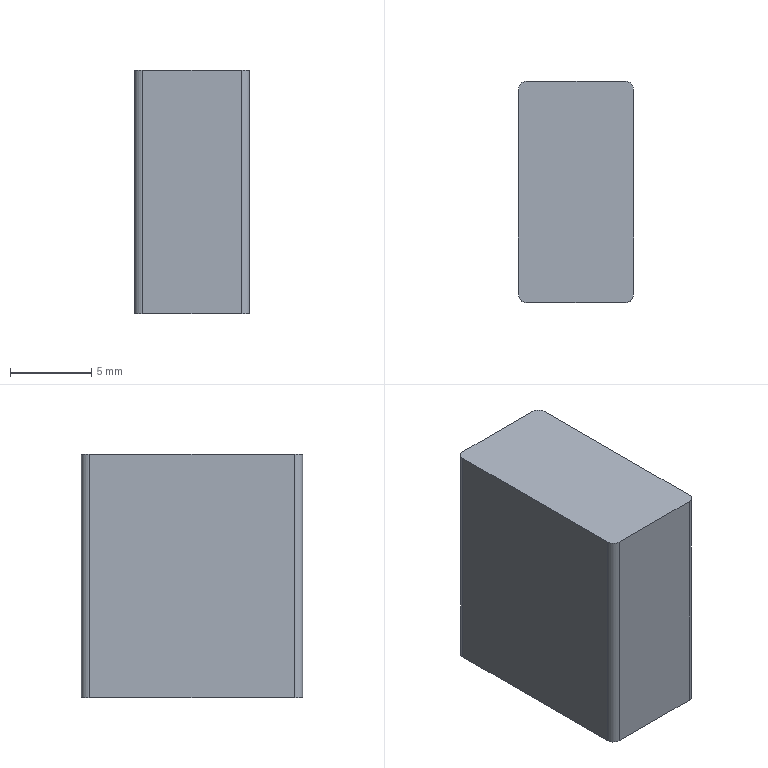Part | NX | features BREP 1 | 1 solid | 10 faces | box 7.1 x 13.637 x 15 mm | volume 1449 mm3 | plane 6 | cylinder 4 | commonest cylinder face diameters 1 x4
STEP:
#1=CARTESIAN_POINT('',(-3.05,6.819,-25.6));
#2=VERTEX_POINT('',#1);
#3=CARTESIAN_POINT('',(-3.55,6.319,-25.6));
#4=VERTEX_POINT('',#3);
#5=CARTESIAN_POINT('',(-3.05,6.319,-25.6));
#6=DIRECTION('',(0.,0.,1.));
#7=DIRECTION('',(1.,0.,0.));
#8=AXIS2_PLACEMENT_3D('',#5,#6,#7);
#9=CIRCLE('',#8,0.5);
#10=EDGE_CURVE('',#2,#4,#9,.T.);
#11=ORIENTED_EDGE('',*,*,#10,.F.);
#12=CARTESIAN_POINT('',(-3.05,6.819,-40.6));
#13=VERTEX_POINT('',#12);
#14=CARTESIAN_POINT('',(-3.05,6.819,-40.6));
#15=DIRECTION('',(0.,0.,1.));
#16=VECTOR('',#15,1000.);
#17=LINE('',#14,#16);
#18=EDGE_CURVE('',#13,#2,#17,.T.);
#19=ORIENTED_EDGE('',*,*,#18,.F.);
#20=CARTESIAN_POINT('',(-3.55,6.319,-40.6));
#21=VERTEX_POINT('',#20);
#22=CARTESIAN_POINT('',(-3.05,6.319,-40.6));
#23=DIRECTION('',(0.,0.,1.));
#24=DIRECTION('',(1.,0.,0.));
#25=AXIS2_PLACEMENT_3D('',#22,#23,#24);
#26=CIRCLE('',#25,0.5);
#27=EDGE_CURVE('',#13,#21,#26,.T.);
#28=ORIENTED_EDGE('',*,*,#27,.T.);
#29=CARTESIAN_POINT('',(-3.55,6.319,-40.6));
#30=DIRECTION('',(0.,0.,1.));
#31=VECTOR('',#30,1000.);
#32=LINE('',#29,#31);
#33=EDGE_CURVE('',#21,#4,#32,.T.);
#34=ORIENTED_EDGE('',*,*,#33,.T.);
#35=EDGE_LOOP('',(#11,#19,#28,#34));
#36=FACE_BOUND('',#35,.T.);
#37=CARTESIAN_POINT('',(-3.05,6.319,-40.6));
#38=DIRECTION('',(0.,0.,1.));
#39=DIRECTION('',(-1.,0.,0.));
#40=AXIS2_PLACEMENT_3D('',#37,#38,#39);
#41=CYLINDRICAL_SURFACE('',#40,0.5);
#42=ADVANCED_FACE('',(#36),#41,.T.);
#43=CARTESIAN_POINT('',(-3.55,-6.319,-25.6));
#44=VERTEX_POINT('',#43);
#45=CARTESIAN_POINT('',(-3.55,-6.319,-25.6));
#46=DIRECTION('',(0.,1.,0.));
#47=VECTOR('',#46,1000.);
#48=LINE('',#45,#47);
#49=EDGE_CURVE('',#44,#4,#48,.T.);
#50=ORIENTED_EDGE('',*,*,#49,.T.);
#51=ORIENTED_EDGE('',*,*,#33,.F.);
#52=CARTESIAN_POINT('',(-3.55,-6.319,-40.6));
#53=VERTEX_POINT('',#52);
#54=CARTESIAN_POINT('',(-3.55,-6.319,-40.6));
#55=DIRECTION('',(0.,1.,0.));
#56=VECTOR('',#55,1000.);
#57=LINE('',#54,#56);
#58=EDGE_CURVE('',#53,#21,#57,.T.);
#59=ORIENTED_EDGE('',*,*,#58,.F.);
#60=CARTESIAN_POINT('',(-3.55,-6.319,-40.6));
#61=DIRECTION('',(0.,0.,1.));
#62=VECTOR('',#61,1000.);
#63=LINE('',#60,#62);
#64=EDGE_CURVE('',#53,#44,#63,.T.);
#65=ORIENTED_EDGE('',*,*,#64,.T.);
#66=EDGE_LOOP('',(#50,#51,#59,#65));
#67=FACE_BOUND('',#66,.T.);
#68=CARTESIAN_POINT('',(-3.55,-6.319,-40.6));
#69=DIRECTION('',(1.,0.,0.));
#70=DIRECTION('',(0.,-1.,0.));
#71=AXIS2_PLACEMENT_3D('',#68,#69,#70);
#72=PLANE('',#71);
#73=ADVANCED_FACE('',(#67),#72,.F.);
#74=CARTESIAN_POINT('',(-3.05,-6.819,-25.6));
#75=VERTEX_POINT('',#74);
#76=CARTESIAN_POINT('',(-3.05,-6.319,-25.6));
#77=DIRECTION('',(0.,0.,1.));
#78=DIRECTION('',(1.,0.,0.));
#79=AXIS2_PLACEMENT_3D('',#76,#77,#78);
#80=CIRCLE('',#79,0.5);
#81=EDGE_CURVE('',#44,#75,#80,.T.);
#82=ORIENTED_EDGE('',*,*,#81,.F.);
#83=ORIENTED_EDGE('',*,*,#64,.F.);
#84=CARTESIAN_POINT('',(-3.05,-6.819,-40.6));
#85=VERTEX_POINT('',#84);
#86=CARTESIAN_POINT('',(-3.05,-6.319,-40.6));
#87=DIRECTION('',(0.,0.,1.));
#88=DIRECTION('',(1.,0.,0.));
#89=AXIS2_PLACEMENT_3D('',#86,#87,#88);
#90=CIRCLE('',#89,0.5);
#91=EDGE_CURVE('',#53,#85,#90,.T.);
#92=ORIENTED_EDGE('',*,*,#91,.T.);
#93=CARTESIAN_POINT('',(-3.05,-6.819,-40.6));
#94=DIRECTION('',(0.,0.,1.));
#95=VECTOR('',#94,1000.);
#96=LINE('',#93,#95);
#97=EDGE_CURVE('',#85,#75,#96,.T.);
#98=ORIENTED_EDGE('',*,*,#97,.T.);
#99=EDGE_LOOP('',(#82,#83,#92,#98));
#100=FACE_BOUND('',#99,.T.);
#101=CARTESIAN_POINT('',(-3.05,-6.319,-40.6));
#102=DIRECTION('',(0.,0.,1.));
#103=DIRECTION('',(-1.,0.,0.));
#104=AXIS2_PLACEMENT_3D('',#101,#102,#103);
#105=CYLINDRICAL_SURFACE('',#104,0.5);
#106=ADVANCED_FACE('',(#100),#105,.T.);
#107=CARTESIAN_POINT('',(3.05,-6.819,-25.6));
#108=VERTEX_POINT('',#107);
#109=CARTESIAN_POINT('',(3.05,-6.819,-25.6));
#110=DIRECTION('',(-1.,0.,0.));
#111=VECTOR('',#110,1000.);
#112=LINE('',#109,#111);
#113=EDGE_CURVE('',#108,#75,#112,.T.);
#114=ORIENTED_EDGE('',*,*,#113,.T.);
#115=ORIENTED_EDGE('',*,*,#97,.F.);
#116=CARTESIAN_POINT('',(3.05,-6.819,-40.6));
#117=VERTEX_POINT('',#116);
#118=CARTESIAN_POINT('',(3.05,-6.819,-40.6));
#119=DIRECTION('',(-1.,0.,0.));
#120=VECTOR('',#119,1000.);
#121=LINE('',#118,#120);
#122=EDGE_CURVE('',#117,#85,#121,.T.);
#123=ORIENTED_EDGE('',*,*,#122,.F.);
#124=CARTESIAN_POINT('',(3.05,-6.819,-40.6));
#125=DIRECTION('',(0.,0.,1.));
#126=VECTOR('',#125,1000.);
#127=LINE('',#124,#126);
#128=EDGE_CURVE('',#117,#108,#127,.T.);
#129=ORIENTED_EDGE('',*,*,#128,.T.);
#130=EDGE_LOOP('',(#114,#115,#123,#129));
#131=FACE_BOUND('',#130,.T.);
#132=CARTESIAN_POINT('',(3.05,-6.819,-40.6));
#133=DIRECTION('',(0.,1.,0.));
#134=DIRECTION('',(0.,0.,-1.));
#135=AXIS2_PLACEMENT_3D('',#132,#133,#134);
#136=PLANE('',#135);
#137=ADVANCED_FACE('',(#131),#136,.F.);
#138=CARTESIAN_POINT('',(3.55,-6.319,-25.6));
#139=VERTEX_POINT('',#138);
#140=CARTESIAN_POINT('',(3.05,-6.319,-25.6));
#141=DIRECTION('',(0.,0.,1.));
#142=DIRECTION('',(1.,0.,0.));
#143=AXIS2_PLACEMENT_3D('',#140,#141,#142);
#144=CIRCLE('',#143,0.5);
#145=EDGE_CURVE('',#108,#139,#144,.T.);
#146=ORIENTED_EDGE('',*,*,#145,.F.);
#147=ORIENTED_EDGE('',*,*,#128,.F.);
#148=CARTESIAN_POINT('',(3.55,-6.319,-40.6));
#149=VERTEX_POINT('',#148);
#150=CARTESIAN_POINT('',(3.05,-6.319,-40.6));
#151=DIRECTION('',(0.,0.,1.));
#152=DIRECTION('',(1.,0.,0.));
#153=AXIS2_PLACEMENT_3D('',#150,#151,#152);
#154=CIRCLE('',#153,0.5);
#155=EDGE_CURVE('',#117,#149,#154,.T.);
#156=ORIENTED_EDGE('',*,*,#155,.T.);
#157=CARTESIAN_POINT('',(3.55,-6.319,-40.6));
#158=DIRECTION('',(0.,0.,1.));
#159=VECTOR('',#158,1000.);
#160=LINE('',#157,#159);
#161=EDGE_CURVE('',#149,#139,#160,.T.);
#162=ORIENTED_EDGE('',*,*,#161,.T.);
#163=EDGE_LOOP('',(#146,#147,#156,#162));
#164=FACE_BOUND('',#163,.T.);
#165=CARTESIAN_POINT('',(3.05,-6.319,-40.6));
#166=DIRECTION('',(0.,0.,1.));
#167=DIRECTION('',(-1.,0.,0.));
#168=AXIS2_PLACEMENT_3D('',#165,#166,#167);
#169=CYLINDRICAL_SURFACE('',#168,0.5);
#170=ADVANCED_FACE('',(#164),#169,.T.);
#171=CARTESIAN_POINT('',(3.55,6.319,-25.6));
#172=VERTEX_POINT('',#171);
#173=CARTESIAN_POINT('',(3.55,6.319,-25.6));
#174=DIRECTION('',(0.,-1.,0.));
#175=VECTOR('',#174,1000.);
#176=LINE('',#173,#175);
#177=EDGE_CURVE('',#172,#139,#176,.T.);
#178=ORIENTED_EDGE('',*,*,#177,.T.);
#179=ORIENTED_EDGE('',*,*,#161,.F.);
#180=CARTESIAN_POINT('',(3.55,6.319,-40.6));
#181=VERTEX_POINT('',#180);
#182=CARTESIAN_POINT('',(3.55,6.319,-40.6));
#183=DIRECTION('',(0.,-1.,0.));
#184=VECTOR('',#183,1000.);
#185=LINE('',#182,#184);
#186=EDGE_CURVE('',#181,#149,#185,.T.);
#187=ORIENTED_EDGE('',*,*,#186,.F.);
#188=CARTESIAN_POINT('',(3.55,6.319,-40.6));
#189=DIRECTION('',(0.,0.,1.));
#190=VECTOR('',#189,1000.);
#191=LINE('',#188,#190);
#192=EDGE_CURVE('',#181,#172,#191,.T.);
#193=ORIENTED_EDGE('',*,*,#192,.T.);
#194=EDGE_LOOP('',(#178,#179,#187,#193));
#195=FACE_BOUND('',#194,.T.);
#196=CARTESIAN_POINT('',(3.55,6.319,-40.6));
#197=DIRECTION('',(-1.,0.,0.));
#198=DIRECTION('',(0.,1.,0.));
#199=AXIS2_PLACEMENT_3D('',#196,#197,#198);
#200=PLANE('',#199);
#201=ADVANCED_FACE('',(#195),#200,.F.);
#202=CARTESIAN_POINT('',(3.05,6.819,-25.6));
#203=VERTEX_POINT('',#202);
#204=CARTESIAN_POINT('',(3.05,6.319,-25.6));
#205=DIRECTION('',(0.,0.,1.));
#206=DIRECTION('',(1.,0.,0.));
#207=AXIS2_PLACEMENT_3D('',#204,#205,#206);
#208=CIRCLE('',#207,0.5);
#209=EDGE_CURVE('',#172,#203,#208,.T.);
#210=ORIENTED_EDGE('',*,*,#209,.F.);
#211=ORIENTED_EDGE('',*,*,#192,.F.);
#212=CARTESIAN_POINT('',(3.05,6.819,-40.6));
#213=VERTEX_POINT('',#212);
#214=CARTESIAN_POINT('',(3.05,6.319,-40.6));
#215=DIRECTION('',(0.,0.,1.));
#216=DIRECTION('',(1.,0.,0.));
#217=AXIS2_PLACEMENT_3D('',#214,#215,#216);
#218=CIRCLE('',#217,0.5);
#219=EDGE_CURVE('',#181,#213,#218,.T.);
#220=ORIENTED_EDGE('',*,*,#219,.T.);
#221=CARTESIAN_POINT('',(3.05,6.819,-40.6));
#222=DIRECTION('',(0.,0.,1.));
#223=VECTOR('',#222,1000.);
#224=LINE('',#221,#223);
#225=EDGE_CURVE('',#213,#203,#224,.T.);
#226=ORIENTED_EDGE('',*,*,#225,.T.);
#227=EDGE_LOOP('',(#210,#211,#220,#226));
#228=FACE_BOUND('',#227,.T.);
#229=CARTESIAN_POINT('',(3.05,6.319,-40.6));
#230=DIRECTION('',(0.,0.,1.));
#231=DIRECTION('',(-1.,0.,0.));
#232=AXIS2_PLACEMENT_3D('',#229,#230,#231);
#233=CYLINDRICAL_SURFACE('',#232,0.5);
#234=ADVANCED_FACE('',(#228),#233,.T.);
#235=CARTESIAN_POINT('',(-3.05,6.819,-25.6));
#236=DIRECTION('',(1.,0.,0.));
#237=VECTOR('',#236,1000.);
#238=LINE('',#235,#237);
#239=EDGE_CURVE('',#2,#203,#238,.T.);
#240=ORIENTED_EDGE('',*,*,#239,.T.);
#241=ORIENTED_EDGE('',*,*,#225,.F.);
#242=CARTESIAN_POINT('',(-3.05,6.819,-40.6));
#243=DIRECTION('',(1.,0.,0.));
#244=VECTOR('',#243,1000.);
#245=LINE('',#242,#244);
#246=EDGE_CURVE('',#13,#213,#245,.T.);
#247=ORIENTED_EDGE('',*,*,#246,.F.);
#248=ORIENTED_EDGE('',*,*,#18,.T.);
#249=EDGE_LOOP('',(#240,#241,#247,#248));
#250=FACE_BOUND('',#249,.T.);
#251=CARTESIAN_POINT('',(-3.05,6.819,-40.6));
#252=DIRECTION('',(0.,-1.,0.));
#253=DIRECTION('',(0.,0.,1.));
#254=AXIS2_PLACEMENT_3D('',#251,#252,#253);
#255=PLANE('',#254);
#256=ADVANCED_FACE('',(#250),#255,.F.);
#257=ORIENTED_EDGE('',*,*,#27,.F.);
#258=ORIENTED_EDGE('',*,*,#246,.T.);
#259=ORIENTED_EDGE('',*,*,#219,.F.);
#260=ORIENTED_EDGE('',*,*,#186,.T.);
#261=ORIENTED_EDGE('',*,*,#155,.F.);
#262=ORIENTED_EDGE('',*,*,#122,.T.);
#263=ORIENTED_EDGE('',*,*,#91,.F.);
#264=ORIENTED_EDGE('',*,*,#58,.T.);
#265=EDGE_LOOP('',(#257,#258,#259,#260,#261,#262,#263,#264));
#266=FACE_BOUND('',#265,.T.);
#267=CARTESIAN_POINT('',(-3.05,6.319,-40.6));
#268=DIRECTION('',(0.,0.,1.));
#269=DIRECTION('',(-1.,0.,0.));
#270=AXIS2_PLACEMENT_3D('',#267,#268,#269);
#271=PLANE('',#270);
#272=ADVANCED_FACE('',(#266),#271,.F.);
#273=ORIENTED_EDGE('',*,*,#10,.T.);
#274=ORIENTED_EDGE('',*,*,#49,.F.);
#275=ORIENTED_EDGE('',*,*,#81,.T.);
#276=ORIENTED_EDGE('',*,*,#113,.F.);
#277=ORIENTED_EDGE('',*,*,#145,.T.);
#278=ORIENTED_EDGE('',*,*,#177,.F.);
#279=ORIENTED_EDGE('',*,*,#209,.T.);
#280=ORIENTED_EDGE('',*,*,#239,.F.);
#281=EDGE_LOOP('',(#273,#274,#275,#276,#277,#278,#279,#280));
#282=FACE_BOUND('',#281,.T.);
#283=CARTESIAN_POINT('',(-3.05,6.319,-25.6));
#284=DIRECTION('',(0.,0.,1.));
#285=DIRECTION('',(-1.,0.,0.));
#286=AXIS2_PLACEMENT_3D('',#283,#284,#285);
#287=PLANE('',#286);
#288=ADVANCED_FACE('',(#282),#287,.T.);
#289=CLOSED_SHELL('',(#42,#73,#106,#137,#170,#201,#234,#256,#272,#288));
#290=MANIFOLD_SOLID_BREP('',#289);
#291=(LENGTH_UNIT()NAMED_UNIT(*)SI_UNIT(.MILLI.,.METRE.));
#292=UNCERTAINTY_MEASURE_WITH_UNIT(LENGTH_MEASURE(0.00001),#291,'','');
#293=(NAMED_UNIT(*)PLANE_ANGLE_UNIT()SI_UNIT($,.RADIAN.));
#294=(NAMED_UNIT(*)SI_UNIT($,.STERADIAN.)SOLID_ANGLE_UNIT());
#295=(GEOMETRIC_REPRESENTATION_CONTEXT(3)GLOBAL_UNCERTAINTY_ASSIGNED_CONTEXT((#292))GLOBAL_UNIT_ASSIGNED_CONTEXT((#291,#293,#294))REPRESENTATION_CONTEXT('',''));
#296=ADVANCED_BREP_SHAPE_REPRESENTATION('',(#290),#295);